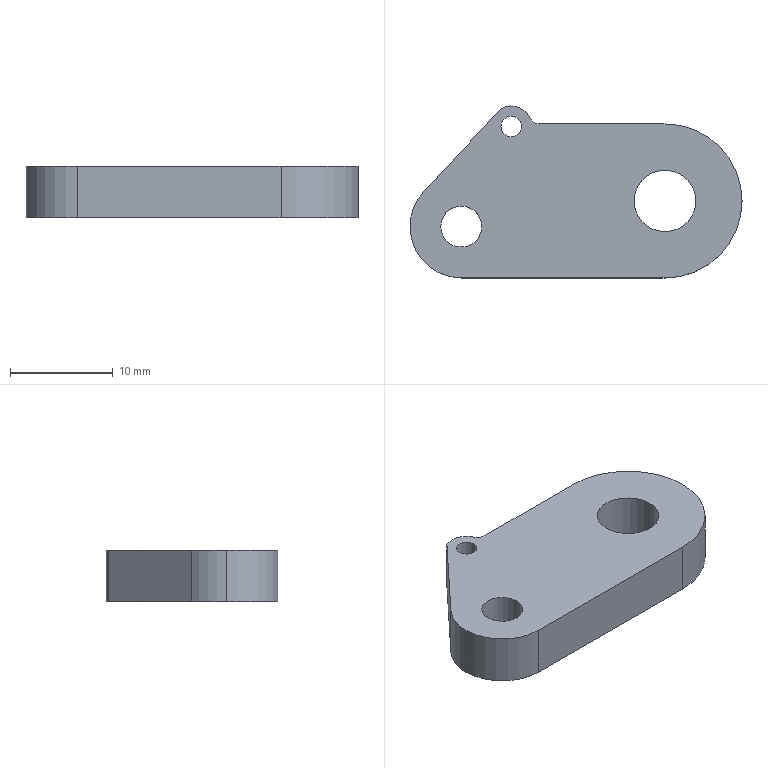Part | SolidWorks | features Extrusion 1 | 1 solid | 16 faces | box 32.34 x 16.75 x 5 mm | volume 1932 mm3 | cylinder 11 | plane 5 | commonest cylinder face diameters 2 x3 4 x3 6 x2 10 x2 15 x1
STEP:
#1=CARTESIAN_POINT('',(-21.84,-2.5,5.));
#2=VERTEX_POINT('',#1);
#3=CARTESIAN_POINT('',(-17.84,-2.5,5.));
#4=VERTEX_POINT('',#3);
#5=CARTESIAN_POINT('',(-19.84,-2.5,5.));
#6=DIRECTION('',(0.,0.,1.));
#7=DIRECTION('',(1.,0.,0.));
#8=AXIS2_PLACEMENT_3D('',#5,#6,#7);
#9=CIRCLE('',#8,2.);
#10=EDGE_CURVE('',#2,#4,#9,.T.);
#11=ORIENTED_EDGE('',*,*,#10,.T.);
#12=CARTESIAN_POINT('',(-17.84,-2.5,0.));
#13=VERTEX_POINT('',#12);
#14=CARTESIAN_POINT('',(-17.84,-2.5,5.));
#15=DIRECTION('',(0.,0.,-1.));
#16=VECTOR('',#15,1000.);
#17=LINE('',#14,#16);
#18=EDGE_CURVE('',#4,#13,#17,.T.);
#19=ORIENTED_EDGE('',*,*,#18,.T.);
#20=CARTESIAN_POINT('',(-21.84,-2.5,0.));
#21=VERTEX_POINT('',#20);
#22=CARTESIAN_POINT('',(-19.84,-2.5,0.));
#23=DIRECTION('',(0.,0.,1.));
#24=DIRECTION('',(1.,0.,0.));
#25=AXIS2_PLACEMENT_3D('',#22,#23,#24);
#26=CIRCLE('',#25,2.);
#27=EDGE_CURVE('',#21,#13,#26,.T.);
#28=ORIENTED_EDGE('',*,*,#27,.F.);
#29=CARTESIAN_POINT('',(-21.84,-2.5,5.));
#30=DIRECTION('',(0.,0.,-1.));
#31=VECTOR('',#30,1000.);
#32=LINE('',#29,#31);
#33=EDGE_CURVE('',#2,#21,#32,.T.);
#34=ORIENTED_EDGE('',*,*,#33,.F.);
#35=EDGE_LOOP('',(#11,#19,#28,#34));
#36=FACE_OUTER_BOUND('',#35,.T.);
#37=CARTESIAN_POINT('',(-19.84,-2.5,5.));
#38=DIRECTION('',(0.,0.,-1.));
#39=DIRECTION('',(-1.,0.,0.));
#40=AXIS2_PLACEMENT_3D('',#37,#38,#39);
#41=CYLINDRICAL_SURFACE('',#40,2.);
#42=ADVANCED_FACE('',(#36),#41,.F.);
#43=CARTESIAN_POINT('',(-15.98,7.25,5.));
#44=VERTEX_POINT('',#43);
#45=CARTESIAN_POINT('',(-13.98,7.25,5.));
#46=VERTEX_POINT('',#45);
#47=CARTESIAN_POINT('',(-14.98,7.25,5.));
#48=DIRECTION('',(0.,0.,1.));
#49=DIRECTION('',(1.,0.,0.));
#50=AXIS2_PLACEMENT_3D('',#47,#48,#49);
#51=CIRCLE('',#50,1.);
#52=EDGE_CURVE('',#44,#46,#51,.T.);
#53=ORIENTED_EDGE('',*,*,#52,.T.);
#54=CARTESIAN_POINT('',(-13.98,7.25,0.));
#55=VERTEX_POINT('',#54);
#56=CARTESIAN_POINT('',(-13.98,7.25,5.));
#57=DIRECTION('',(0.,0.,-1.));
#58=VECTOR('',#57,1000.);
#59=LINE('',#56,#58);
#60=EDGE_CURVE('',#46,#55,#59,.T.);
#61=ORIENTED_EDGE('',*,*,#60,.T.);
#62=CARTESIAN_POINT('',(-15.98,7.25,0.));
#63=VERTEX_POINT('',#62);
#64=CARTESIAN_POINT('',(-14.98,7.25,0.));
#65=DIRECTION('',(0.,0.,1.));
#66=DIRECTION('',(1.,0.,0.));
#67=AXIS2_PLACEMENT_3D('',#64,#65,#66);
#68=CIRCLE('',#67,1.);
#69=EDGE_CURVE('',#63,#55,#68,.T.);
#70=ORIENTED_EDGE('',*,*,#69,.F.);
#71=CARTESIAN_POINT('',(-15.98,7.25,5.));
#72=DIRECTION('',(0.,0.,-1.));
#73=VECTOR('',#72,1000.);
#74=LINE('',#71,#73);
#75=EDGE_CURVE('',#44,#63,#74,.T.);
#76=ORIENTED_EDGE('',*,*,#75,.F.);
#77=EDGE_LOOP('',(#53,#61,#70,#76));
#78=FACE_OUTER_BOUND('',#77,.T.);
#79=CARTESIAN_POINT('',(-14.98,7.25,5.));
#80=DIRECTION('',(0.,0.,-1.));
#81=DIRECTION('',(-1.,0.,0.));
#82=AXIS2_PLACEMENT_3D('',#79,#80,#81);
#83=CYLINDRICAL_SURFACE('',#82,1.);
#84=ADVANCED_FACE('',(#78),#83,.F.);
#85=CARTESIAN_POINT('',(-3.,0.,5.));
#86=VERTEX_POINT('',#85);
#87=CARTESIAN_POINT('',(3.,0.,5.));
#88=VERTEX_POINT('',#87);
#89=CARTESIAN_POINT('',(0.,0.,5.));
#90=DIRECTION('',(0.,0.,1.));
#91=DIRECTION('',(1.,0.,0.));
#92=AXIS2_PLACEMENT_3D('',#89,#90,#91);
#93=CIRCLE('',#92,3.);
#94=EDGE_CURVE('',#86,#88,#93,.T.);
#95=ORIENTED_EDGE('',*,*,#94,.T.);
#96=CARTESIAN_POINT('',(3.,0.,0.));
#97=VERTEX_POINT('',#96);
#98=CARTESIAN_POINT('',(3.,0.,5.));
#99=DIRECTION('',(0.,0.,-1.));
#100=VECTOR('',#99,1000.);
#101=LINE('',#98,#100);
#102=EDGE_CURVE('',#88,#97,#101,.T.);
#103=ORIENTED_EDGE('',*,*,#102,.T.);
#104=CARTESIAN_POINT('',(-3.,0.,0.));
#105=VERTEX_POINT('',#104);
#106=CARTESIAN_POINT('',(0.,0.,0.));
#107=DIRECTION('',(0.,0.,1.));
#108=DIRECTION('',(1.,0.,0.));
#109=AXIS2_PLACEMENT_3D('',#106,#107,#108);
#110=CIRCLE('',#109,3.);
#111=EDGE_CURVE('',#105,#97,#110,.T.);
#112=ORIENTED_EDGE('',*,*,#111,.F.);
#113=CARTESIAN_POINT('',(-3.,0.,5.));
#114=DIRECTION('',(0.,0.,-1.));
#115=VECTOR('',#114,1000.);
#116=LINE('',#113,#115);
#117=EDGE_CURVE('',#86,#105,#116,.T.);
#118=ORIENTED_EDGE('',*,*,#117,.F.);
#119=EDGE_LOOP('',(#95,#103,#112,#118));
#120=FACE_OUTER_BOUND('',#119,.T.);
#121=CARTESIAN_POINT('',(0.,0.,5.));
#122=DIRECTION('',(0.,0.,-1.));
#123=DIRECTION('',(-1.,0.,0.));
#124=AXIS2_PLACEMENT_3D('',#121,#122,#123);
#125=CYLINDRICAL_SURFACE('',#124,3.);
#126=ADVANCED_FACE('',(#120),#125,.F.);
#127=CARTESIAN_POINT('',(-24.84,-2.5,5.));
#128=VERTEX_POINT('',#127);
#129=CARTESIAN_POINT('',(-19.84,-7.5,5.));
#130=VERTEX_POINT('',#129);
#131=CARTESIAN_POINT('',(-19.84,-2.5,5.));
#132=DIRECTION('',(0.,0.,1.));
#133=DIRECTION('',(1.,0.,0.));
#134=AXIS2_PLACEMENT_3D('',#131,#132,#133);
#135=CIRCLE('',#134,5.);
#136=EDGE_CURVE('',#128,#130,#135,.T.);
#137=ORIENTED_EDGE('',*,*,#136,.F.);
#138=CARTESIAN_POINT('',(-24.84,-2.5,0.));
#139=VERTEX_POINT('',#138);
#140=CARTESIAN_POINT('',(-24.84,-2.5,5.));
#141=DIRECTION('',(0.,0.,-1.));
#142=VECTOR('',#141,1000.);
#143=LINE('',#140,#142);
#144=EDGE_CURVE('',#128,#139,#143,.T.);
#145=ORIENTED_EDGE('',*,*,#144,.T.);
#146=CARTESIAN_POINT('',(-19.84,-7.5,0.));
#147=VERTEX_POINT('',#146);
#148=CARTESIAN_POINT('',(-19.84,-2.5,0.));
#149=DIRECTION('',(0.,0.,1.));
#150=DIRECTION('',(1.,0.,0.));
#151=AXIS2_PLACEMENT_3D('',#148,#149,#150);
#152=CIRCLE('',#151,5.);
#153=EDGE_CURVE('',#139,#147,#152,.T.);
#154=ORIENTED_EDGE('',*,*,#153,.T.);
#155=CARTESIAN_POINT('',(-19.84,-7.5,5.));
#156=DIRECTION('',(0.,0.,-1.));
#157=VECTOR('',#156,1000.);
#158=LINE('',#155,#157);
#159=EDGE_CURVE('',#130,#147,#158,.T.);
#160=ORIENTED_EDGE('',*,*,#159,.F.);
#161=EDGE_LOOP('',(#137,#145,#154,#160));
#162=FACE_OUTER_BOUND('',#161,.T.);
#163=CARTESIAN_POINT('',(-19.84,-2.5,5.));
#164=DIRECTION('',(0.,0.,-1.));
#165=DIRECTION('',(-1.,0.,0.));
#166=AXIS2_PLACEMENT_3D('',#163,#164,#165);
#167=CYLINDRICAL_SURFACE('',#166,5.);
#168=ADVANCED_FACE('',(#162),#167,.T.);
#169=ORIENTED_EDGE('',*,*,#52,.F.);
#170=CARTESIAN_POINT('',(-14.98,7.25,5.));
#171=DIRECTION('',(0.,0.,1.));
#172=DIRECTION('',(1.,0.,0.));
#173=AXIS2_PLACEMENT_3D('',#170,#171,#172);
#174=CIRCLE('',#173,1.);
#175=EDGE_CURVE('',#46,#44,#174,.T.);
#176=ORIENTED_EDGE('',*,*,#175,.F.);
#177=EDGE_LOOP('',(#169,#176));
#178=FACE_BOUND('',#177,.T.);
#179=CARTESIAN_POINT('',(-12.253,7.5,5.));
#180=VERTEX_POINT('',#179);
#181=CARTESIAN_POINT('',(-13.162,8.083,5.));
#182=VERTEX_POINT('',#181);
#183=CARTESIAN_POINT('',(-12.253,8.5,5.));
#184=DIRECTION('',(0.,0.,-1.));
#185=DIRECTION('',(1.,0.,0.));
#186=AXIS2_PLACEMENT_3D('',#183,#184,#185);
#187=CIRCLE('',#186,1.);
#188=EDGE_CURVE('',#180,#182,#187,.T.);
#189=ORIENTED_EDGE('',*,*,#188,.T.);
#190=CARTESIAN_POINT('',(-15.958,8.995,5.));
#191=VERTEX_POINT('',#190);
#192=CARTESIAN_POINT('',(-14.98,7.25,5.));
#193=DIRECTION('',(0.,0.,1.));
#194=DIRECTION('',(1.,0.,0.));
#195=AXIS2_PLACEMENT_3D('',#192,#193,#194);
#196=CIRCLE('',#195,2.);
#197=EDGE_CURVE('',#182,#191,#196,.T.);
#198=ORIENTED_EDGE('',*,*,#197,.T.);
#199=CARTESIAN_POINT('',(-23.497,0.91,5.));
#200=VERTEX_POINT('',#199);
#201=CARTESIAN_POINT('',(-15.958,8.995,5.));
#202=DIRECTION('',(-0.682,-0.7314,0.));
#203=VECTOR('',#202,1000.);
#204=LINE('',#201,#203);
#205=EDGE_CURVE('',#191,#200,#204,.T.);
#206=ORIENTED_EDGE('',*,*,#205,.T.);
#207=CARTESIAN_POINT('',(-19.84,-2.5,5.));
#208=DIRECTION('',(0.,0.,1.));
#209=DIRECTION('',(1.,0.,0.));
#210=AXIS2_PLACEMENT_3D('',#207,#208,#209);
#211=CIRCLE('',#210,5.);
#212=EDGE_CURVE('',#200,#128,#211,.T.);
#213=ORIENTED_EDGE('',*,*,#212,.T.);
#214=ORIENTED_EDGE('',*,*,#136,.T.);
#215=CARTESIAN_POINT('',(0.,-7.5,5.));
#216=VERTEX_POINT('',#215);
#217=CARTESIAN_POINT('',(-19.84,-7.5,5.));
#218=DIRECTION('',(1.,0.,0.));
#219=VECTOR('',#218,1000.);
#220=LINE('',#217,#219);
#221=EDGE_CURVE('',#130,#216,#220,.T.);
#222=ORIENTED_EDGE('',*,*,#221,.T.);
#223=CARTESIAN_POINT('',(0.,7.5,5.));
#224=VERTEX_POINT('',#223);
#225=CARTESIAN_POINT('',(0.,0.,5.));
#226=DIRECTION('',(0.,0.,1.));
#227=DIRECTION('',(1.,0.,0.));
#228=AXIS2_PLACEMENT_3D('',#225,#226,#227);
#229=CIRCLE('',#228,7.5);
#230=EDGE_CURVE('',#216,#224,#229,.T.);
#231=ORIENTED_EDGE('',*,*,#230,.T.);
#232=CARTESIAN_POINT('',(0.,7.5,5.));
#233=DIRECTION('',(-1.,0.,0.));
#234=VECTOR('',#233,1000.);
#235=LINE('',#232,#234);
#236=EDGE_CURVE('',#224,#180,#235,.T.);
#237=ORIENTED_EDGE('',*,*,#236,.T.);
#238=EDGE_LOOP('',(#189,#198,#206,#213,#214,#222,#231,#237));
#239=FACE_OUTER_BOUND('',#238,.T.);
#240=ORIENTED_EDGE('',*,*,#94,.F.);
#241=CARTESIAN_POINT('',(0.,0.,5.));
#242=DIRECTION('',(0.,0.,1.));
#243=DIRECTION('',(1.,0.,0.));
#244=AXIS2_PLACEMENT_3D('',#241,#242,#243);
#245=CIRCLE('',#244,3.);
#246=EDGE_CURVE('',#88,#86,#245,.T.);
#247=ORIENTED_EDGE('',*,*,#246,.F.);
#248=EDGE_LOOP('',(#240,#247));
#249=FACE_BOUND('',#248,.T.);
#250=ORIENTED_EDGE('',*,*,#10,.F.);
#251=CARTESIAN_POINT('',(-19.84,-2.5,5.));
#252=DIRECTION('',(0.,0.,1.));
#253=DIRECTION('',(1.,0.,0.));
#254=AXIS2_PLACEMENT_3D('',#251,#252,#253);
#255=CIRCLE('',#254,2.);
#256=EDGE_CURVE('',#4,#2,#255,.T.);
#257=ORIENTED_EDGE('',*,*,#256,.F.);
#258=EDGE_LOOP('',(#250,#257));
#259=FACE_BOUND('',#258,.T.);
#260=CARTESIAN_POINT('',(-12.253,8.5,5.));
#261=DIRECTION('',(0.,0.,1.));
#262=DIRECTION('',(1.,0.,0.));
#263=AXIS2_PLACEMENT_3D('',#260,#261,#262);
#264=PLANE('',#263);
#265=ADVANCED_FACE('',(#178,#239,#249,#259),#264,.T.);
#266=CARTESIAN_POINT('',(-12.253,7.5,0.));
#267=VERTEX_POINT('',#266);
#268=CARTESIAN_POINT('',(-13.162,8.083,0.));
#269=VERTEX_POINT('',#268);
#270=CARTESIAN_POINT('',(-12.253,8.5,0.));
#271=DIRECTION('',(0.,0.,-1.));
#272=DIRECTION('',(1.,0.,0.));
#273=AXIS2_PLACEMENT_3D('',#270,#271,#272);
#274=CIRCLE('',#273,1.);
#275=EDGE_CURVE('',#267,#269,#274,.T.);
#276=ORIENTED_EDGE('',*,*,#275,.F.);
#277=CARTESIAN_POINT('',(0.,7.5,0.));
#278=VERTEX_POINT('',#277);
#279=CARTESIAN_POINT('',(0.,7.5,0.));
#280=DIRECTION('',(-1.,0.,0.));
#281=VECTOR('',#280,1000.);
#282=LINE('',#279,#281);
#283=EDGE_CURVE('',#278,#267,#282,.T.);
#284=ORIENTED_EDGE('',*,*,#283,.F.);
#285=CARTESIAN_POINT('',(0.,-7.5,0.));
#286=VERTEX_POINT('',#285);
#287=CARTESIAN_POINT('',(0.,0.,0.));
#288=DIRECTION('',(0.,0.,1.));
#289=DIRECTION('',(1.,0.,0.));
#290=AXIS2_PLACEMENT_3D('',#287,#288,#289);
#291=CIRCLE('',#290,7.5);
#292=EDGE_CURVE('',#286,#278,#291,.T.);
#293=ORIENTED_EDGE('',*,*,#292,.F.);
#294=CARTESIAN_POINT('',(-19.84,-7.5,0.));
#295=DIRECTION('',(1.,0.,0.));
#296=VECTOR('',#295,1000.);
#297=LINE('',#294,#296);
#298=EDGE_CURVE('',#147,#286,#297,.T.);
#299=ORIENTED_EDGE('',*,*,#298,.F.);
#300=ORIENTED_EDGE('',*,*,#153,.F.);
#301=CARTESIAN_POINT('',(-23.497,0.91,0.));
#302=VERTEX_POINT('',#301);
#303=CARTESIAN_POINT('',(-19.84,-2.5,0.));
#304=DIRECTION('',(0.,0.,1.));
#305=DIRECTION('',(1.,0.,0.));
#306=AXIS2_PLACEMENT_3D('',#303,#304,#305);
#307=CIRCLE('',#306,5.);
#308=EDGE_CURVE('',#302,#139,#307,.T.);
#309=ORIENTED_EDGE('',*,*,#308,.F.);
#310=CARTESIAN_POINT('',(-15.958,8.995,0.));
#311=VERTEX_POINT('',#310);
#312=CARTESIAN_POINT('',(-15.958,8.995,0.));
#313=DIRECTION('',(-0.682,-0.7314,0.));
#314=VECTOR('',#313,1000.);
#315=LINE('',#312,#314);
#316=EDGE_CURVE('',#311,#302,#315,.T.);
#317=ORIENTED_EDGE('',*,*,#316,.F.);
#318=CARTESIAN_POINT('',(-14.98,7.25,0.));
#319=DIRECTION('',(0.,0.,1.));
#320=DIRECTION('',(1.,0.,0.));
#321=AXIS2_PLACEMENT_3D('',#318,#319,#320);
#322=CIRCLE('',#321,2.);
#323=EDGE_CURVE('',#269,#311,#322,.T.);
#324=ORIENTED_EDGE('',*,*,#323,.F.);
#325=EDGE_LOOP('',(#276,#284,#293,#299,#300,#309,#317,#324));
#326=FACE_OUTER_BOUND('',#325,.T.);
#327=ORIENTED_EDGE('',*,*,#111,.T.);
#328=CARTESIAN_POINT('',(0.,0.,0.));
#329=DIRECTION('',(0.,0.,1.));
#330=DIRECTION('',(1.,0.,0.));
#331=AXIS2_PLACEMENT_3D('',#328,#329,#330);
#332=CIRCLE('',#331,3.);
#333=EDGE_CURVE('',#97,#105,#332,.T.);
#334=ORIENTED_EDGE('',*,*,#333,.T.);
#335=EDGE_LOOP('',(#327,#334));
#336=FACE_BOUND('',#335,.T.);
#337=ORIENTED_EDGE('',*,*,#69,.T.);
#338=CARTESIAN_POINT('',(-14.98,7.25,0.));
#339=DIRECTION('',(0.,0.,1.));
#340=DIRECTION('',(1.,0.,0.));
#341=AXIS2_PLACEMENT_3D('',#338,#339,#340);
#342=CIRCLE('',#341,1.);
#343=EDGE_CURVE('',#55,#63,#342,.T.);
#344=ORIENTED_EDGE('',*,*,#343,.T.);
#345=EDGE_LOOP('',(#337,#344));
#346=FACE_BOUND('',#345,.T.);
#347=ORIENTED_EDGE('',*,*,#27,.T.);
#348=CARTESIAN_POINT('',(-19.84,-2.5,0.));
#349=DIRECTION('',(0.,0.,1.));
#350=DIRECTION('',(1.,0.,0.));
#351=AXIS2_PLACEMENT_3D('',#348,#349,#350);
#352=CIRCLE('',#351,2.);
#353=EDGE_CURVE('',#13,#21,#352,.T.);
#354=ORIENTED_EDGE('',*,*,#353,.T.);
#355=EDGE_LOOP('',(#347,#354));
#356=FACE_BOUND('',#355,.T.);
#357=CARTESIAN_POINT('',(-12.253,8.5,0.));
#358=DIRECTION('',(0.,0.,1.));
#359=DIRECTION('',(1.,0.,0.));
#360=AXIS2_PLACEMENT_3D('',#357,#358,#359);
#361=PLANE('',#360);
#362=ADVANCED_FACE('',(#326,#336,#346,#356),#361,.F.);
#363=ORIENTED_EDGE('',*,*,#275,.T.);
#364=CARTESIAN_POINT('',(-13.162,8.083,5.));
#365=DIRECTION('',(0.,0.,-1.));
#366=VECTOR('',#365,1000.);
#367=LINE('',#364,#366);
#368=EDGE_CURVE('',#182,#269,#367,.T.);
#369=ORIENTED_EDGE('',*,*,#368,.F.);
#370=ORIENTED_EDGE('',*,*,#188,.F.);
#371=CARTESIAN_POINT('',(-12.253,7.5,5.));
#372=DIRECTION('',(0.,0.,-1.));
#373=VECTOR('',#372,1000.);
#374=LINE('',#371,#373);
#375=EDGE_CURVE('',#180,#267,#374,.T.);
#376=ORIENTED_EDGE('',*,*,#375,.T.);
#377=EDGE_LOOP('',(#363,#369,#370,#376));
#378=FACE_OUTER_BOUND('',#377,.T.);
#379=CARTESIAN_POINT('',(-12.253,8.5,5.));
#380=DIRECTION('',(0.,0.,-1.));
#381=DIRECTION('',(-1.,0.,0.));
#382=AXIS2_PLACEMENT_3D('',#379,#380,#381);
#383=CYLINDRICAL_SURFACE('',#382,1.);
#384=ADVANCED_FACE('',(#378),#383,.F.);
#385=ORIENTED_EDGE('',*,*,#323,.T.);
#386=CARTESIAN_POINT('',(-15.958,8.995,5.));
#387=DIRECTION('',(0.,0.,-1.));
#388=VECTOR('',#387,1000.);
#389=LINE('',#386,#388);
#390=EDGE_CURVE('',#191,#311,#389,.T.);
#391=ORIENTED_EDGE('',*,*,#390,.F.);
#392=ORIENTED_EDGE('',*,*,#197,.F.);
#393=ORIENTED_EDGE('',*,*,#368,.T.);
#394=EDGE_LOOP('',(#385,#391,#392,#393));
#395=FACE_OUTER_BOUND('',#394,.T.);
#396=CARTESIAN_POINT('',(-14.98,7.25,5.));
#397=DIRECTION('',(0.,0.,-1.));
#398=DIRECTION('',(-1.,0.,0.));
#399=AXIS2_PLACEMENT_3D('',#396,#397,#398);
#400=CYLINDRICAL_SURFACE('',#399,2.);
#401=ADVANCED_FACE('',(#395),#400,.T.);
#402=ORIENTED_EDGE('',*,*,#316,.T.);
#403=CARTESIAN_POINT('',(-23.497,0.91,5.));
#404=DIRECTION('',(0.,0.,-1.));
#405=VECTOR('',#404,1000.);
#406=LINE('',#403,#405);
#407=EDGE_CURVE('',#200,#302,#406,.T.);
#408=ORIENTED_EDGE('',*,*,#407,.F.);
#409=ORIENTED_EDGE('',*,*,#205,.F.);
#410=ORIENTED_EDGE('',*,*,#390,.T.);
#411=EDGE_LOOP('',(#402,#408,#409,#410));
#412=FACE_OUTER_BOUND('',#411,.T.);
#413=CARTESIAN_POINT('',(-15.958,8.995,5.));
#414=DIRECTION('',(0.7314,-0.682,0.));
#415=DIRECTION('',(0.682,0.7314,0.));
#416=AXIS2_PLACEMENT_3D('',#413,#414,#415);
#417=PLANE('',#416);
#418=ADVANCED_FACE('',(#412),#417,.F.);
#419=ORIENTED_EDGE('',*,*,#144,.F.);
#420=ORIENTED_EDGE('',*,*,#212,.F.);
#421=ORIENTED_EDGE('',*,*,#407,.T.);
#422=ORIENTED_EDGE('',*,*,#308,.T.);
#423=EDGE_LOOP('',(#419,#420,#421,#422));
#424=FACE_OUTER_BOUND('',#423,.T.);
#425=CARTESIAN_POINT('',(-19.84,-2.5,5.));
#426=DIRECTION('',(0.,0.,-1.));
#427=DIRECTION('',(-1.,0.,0.));
#428=AXIS2_PLACEMENT_3D('',#425,#426,#427);
#429=CYLINDRICAL_SURFACE('',#428,5.);
#430=ADVANCED_FACE('',(#424),#429,.T.);
#431=ORIENTED_EDGE('',*,*,#298,.T.);
#432=CARTESIAN_POINT('',(0.,-7.5,5.));
#433=DIRECTION('',(0.,0.,-1.));
#434=VECTOR('',#433,1000.);
#435=LINE('',#432,#434);
#436=EDGE_CURVE('',#216,#286,#435,.T.);
#437=ORIENTED_EDGE('',*,*,#436,.F.);
#438=ORIENTED_EDGE('',*,*,#221,.F.);
#439=ORIENTED_EDGE('',*,*,#159,.T.);
#440=EDGE_LOOP('',(#431,#437,#438,#439));
#441=FACE_OUTER_BOUND('',#440,.T.);
#442=CARTESIAN_POINT('',(-19.84,-7.5,5.));
#443=DIRECTION('',(0.,1.,0.));
#444=DIRECTION('',(-1.,0.,0.));
#445=AXIS2_PLACEMENT_3D('',#442,#443,#444);
#446=PLANE('',#445);
#447=ADVANCED_FACE('',(#441),#446,.F.);
#448=ORIENTED_EDGE('',*,*,#292,.T.);
#449=CARTESIAN_POINT('',(0.,7.5,5.));
#450=DIRECTION('',(0.,0.,-1.));
#451=VECTOR('',#450,1000.);
#452=LINE('',#449,#451);
#453=EDGE_CURVE('',#224,#278,#452,.T.);
#454=ORIENTED_EDGE('',*,*,#453,.F.);
#455=ORIENTED_EDGE('',*,*,#230,.F.);
#456=ORIENTED_EDGE('',*,*,#436,.T.);
#457=EDGE_LOOP('',(#448,#454,#455,#456));
#458=FACE_OUTER_BOUND('',#457,.T.);
#459=CARTESIAN_POINT('',(0.,0.,5.));
#460=DIRECTION('',(0.,0.,-1.));
#461=DIRECTION('',(-1.,0.,0.));
#462=AXIS2_PLACEMENT_3D('',#459,#460,#461);
#463=CYLINDRICAL_SURFACE('',#462,7.5);
#464=ADVANCED_FACE('',(#458),#463,.T.);
#465=ORIENTED_EDGE('',*,*,#283,.T.);
#466=ORIENTED_EDGE('',*,*,#375,.F.);
#467=ORIENTED_EDGE('',*,*,#236,.F.);
#468=ORIENTED_EDGE('',*,*,#453,.T.);
#469=EDGE_LOOP('',(#465,#466,#467,#468));
#470=FACE_OUTER_BOUND('',#469,.T.);
#471=CARTESIAN_POINT('',(0.,7.5,5.));
#472=DIRECTION('',(0.,-1.,0.));
#473=DIRECTION('',(1.,0.,0.));
#474=AXIS2_PLACEMENT_3D('',#471,#472,#473);
#475=PLANE('',#474);
#476=ADVANCED_FACE('',(#470),#475,.F.);
#477=ORIENTED_EDGE('',*,*,#102,.F.);
#478=ORIENTED_EDGE('',*,*,#246,.T.);
#479=ORIENTED_EDGE('',*,*,#117,.T.);
#480=ORIENTED_EDGE('',*,*,#333,.F.);
#481=EDGE_LOOP('',(#477,#478,#479,#480));
#482=FACE_OUTER_BOUND('',#481,.T.);
#483=CARTESIAN_POINT('',(0.,0.,5.));
#484=DIRECTION('',(0.,0.,-1.));
#485=DIRECTION('',(-1.,0.,0.));
#486=AXIS2_PLACEMENT_3D('',#483,#484,#485);
#487=CYLINDRICAL_SURFACE('',#486,3.);
#488=ADVANCED_FACE('',(#482),#487,.F.);
#489=ORIENTED_EDGE('',*,*,#60,.F.);
#490=ORIENTED_EDGE('',*,*,#175,.T.);
#491=ORIENTED_EDGE('',*,*,#75,.T.);
#492=ORIENTED_EDGE('',*,*,#343,.F.);
#493=EDGE_LOOP('',(#489,#490,#491,#492));
#494=FACE_OUTER_BOUND('',#493,.T.);
#495=CARTESIAN_POINT('',(-14.98,7.25,5.));
#496=DIRECTION('',(0.,0.,-1.));
#497=DIRECTION('',(-1.,0.,0.));
#498=AXIS2_PLACEMENT_3D('',#495,#496,#497);
#499=CYLINDRICAL_SURFACE('',#498,1.);
#500=ADVANCED_FACE('',(#494),#499,.F.);
#501=ORIENTED_EDGE('',*,*,#18,.F.);
#502=ORIENTED_EDGE('',*,*,#256,.T.);
#503=ORIENTED_EDGE('',*,*,#33,.T.);
#504=ORIENTED_EDGE('',*,*,#353,.F.);
#505=EDGE_LOOP('',(#501,#502,#503,#504));
#506=FACE_OUTER_BOUND('',#505,.T.);
#507=CARTESIAN_POINT('',(-19.84,-2.5,5.));
#508=DIRECTION('',(0.,0.,-1.));
#509=DIRECTION('',(-1.,0.,0.));
#510=AXIS2_PLACEMENT_3D('',#507,#508,#509);
#511=CYLINDRICAL_SURFACE('',#510,2.);
#512=ADVANCED_FACE('',(#506),#511,.F.);
#513=CLOSED_SHELL('',(#42,#84,#126,#168,#265,#362,#384,#401,#418,#430,#447,#464,#476,#488,#500,#512));
#514=MANIFOLD_SOLID_BREP('',#513);
#515=CARTESIAN_POINT('',(0.,0.,0.));
#516=DIRECTION('',(0.,0.,1.));
#517=DIRECTION('',(1.,0.,0.));
#518=AXIS2_PLACEMENT_3D('',#515,#516,#517);
#519=(LENGTH_UNIT()NAMED_UNIT(*)SI_UNIT(.MILLI.,.METRE.));
#520=UNCERTAINTY_MEASURE_WITH_UNIT(LENGTH_MEASURE(0.00001),#519,'','');
#521=(NAMED_UNIT(*)PLANE_ANGLE_UNIT()SI_UNIT($,.RADIAN.));
#522=(NAMED_UNIT(*)SI_UNIT($,.STERADIAN.)SOLID_ANGLE_UNIT());
#523=(GEOMETRIC_REPRESENTATION_CONTEXT(3)GLOBAL_UNCERTAINTY_ASSIGNED_CONTEXT((#520))GLOBAL_UNIT_ASSIGNED_CONTEXT((#519,#521,#522))REPRESENTATION_CONTEXT('',''));
#524=ADVANCED_BREP_SHAPE_REPRESENTATION('',(#514,#518),#523);